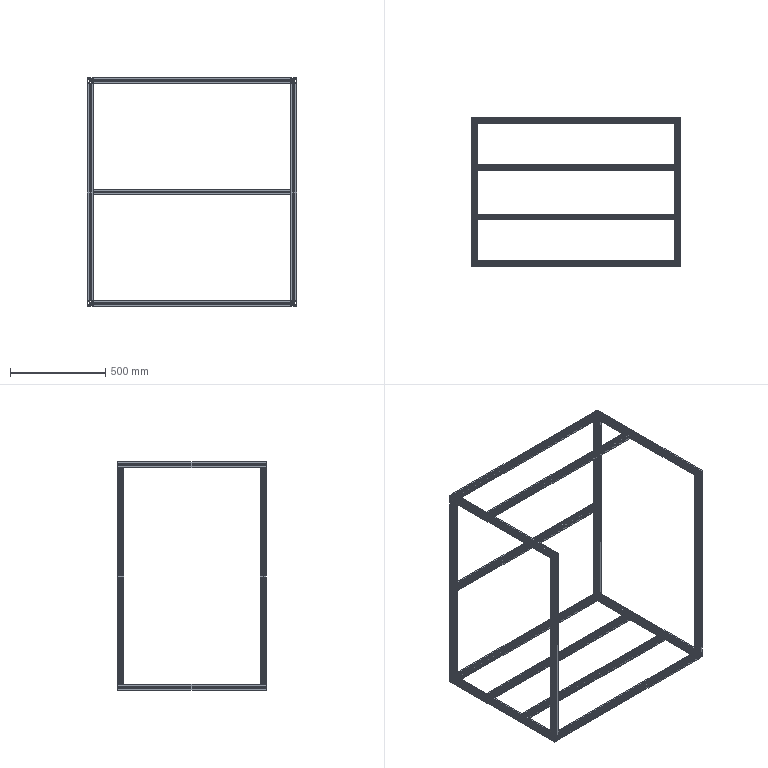Part | SolidWorks | features ICE 14, 3DProfileFeature 2, HoleWzd 2, WeldMemberFeat 2, WeldmentFeature 1 | 15 solids | 1566 faces | box 1100 x 780 x 1200 mm | volume 5922757 mm3 | plane 1084 | cylinder 482 | commonest cylinder face diameters 17.968 x184 6 x120 5 x54 16 x40 12 x28 6.4 x24